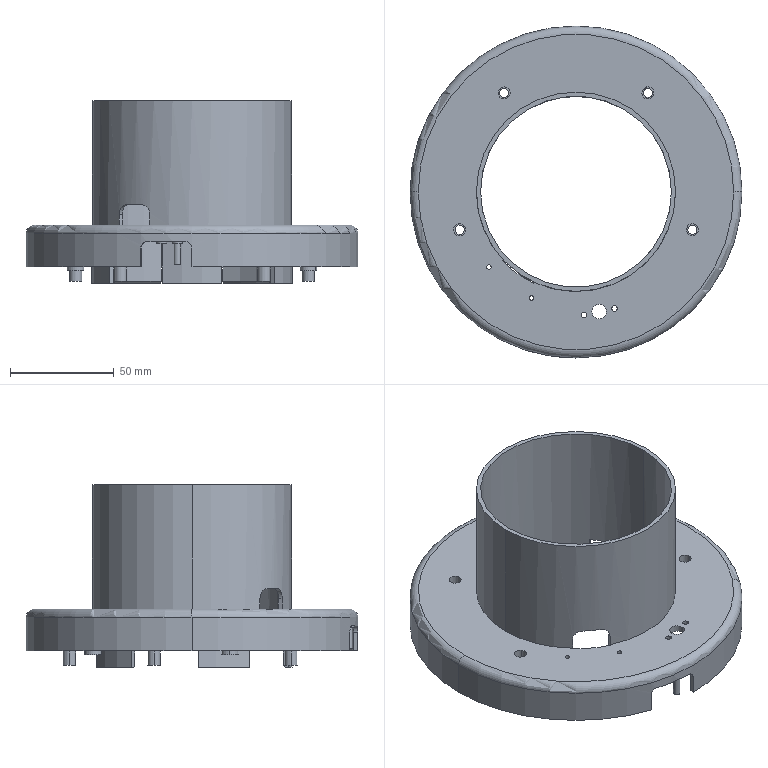Part | SolidWorks | features ICE 20, CirPattern 4, Fillet 4, Chamfer 2, Cut 1, DelFace 1, Extrusion 1 | 1 solid | 263 faces | box 160 x 160 x 88 mm | volume 94016 mm3 | plane 143 | cylinder 84 | torus 27 | cone 9 | commonest cylinder face diameters 6 x12 4.4 x8 5 x8 5.8 x8 8 x8 97 x6